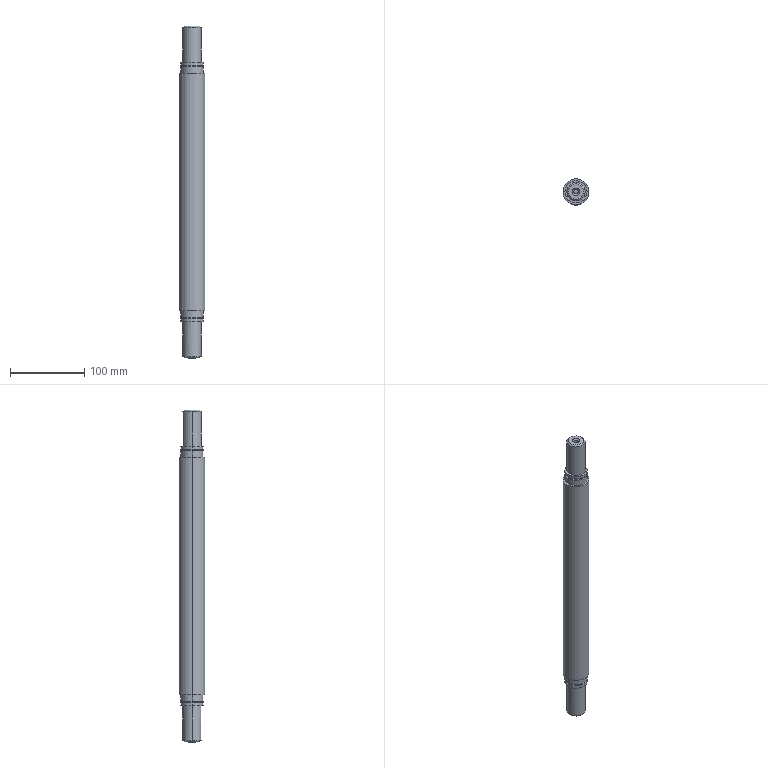Part | STEP file | Shaft 3 | 1 solid | 42 faces | box 35 x 35 x 448 mm | volume 375515 mm3 | cylinder 22 | plane 12 | cone 8 | commonest cylinder face diameters 30 x8 6 x4 25 x4 27.6 x4 35 x2
STEP:
#1=CARTESIAN_POINT('',(-17.5,0.,335.));
#2=VERTEX_POINT('',#1);
#3=CARTESIAN_POINT('',(17.5,0.,335.));
#4=VERTEX_POINT('',#3);
#5=CARTESIAN_POINT('',(0.,0.,335.));
#6=DIRECTION('',(0.,0.,-1.));
#7=DIRECTION('',(-1.,0.,0.));
#8=AXIS2_PLACEMENT_3D('',#5,#6,#7);
#9=CIRCLE('',#8,17.5);
#10=EDGE_CURVE('',#2,#4,#9,.T.);
#11=ORIENTED_EDGE('',*,*,#10,.T.);
#12=CARTESIAN_POINT('',(17.5,0.,15.));
#13=VERTEX_POINT('',#12);
#14=CARTESIAN_POINT('',(17.5,0.,350.));
#15=DIRECTION('',(0.,0.,-1.));
#16=VECTOR('',#15,1000.);
#17=LINE('',#14,#16);
#18=EDGE_CURVE('',#4,#13,#17,.T.);
#19=ORIENTED_EDGE('',*,*,#18,.T.);
#20=CARTESIAN_POINT('',(-17.5,0.,15.));
#21=VERTEX_POINT('',#20);
#22=CARTESIAN_POINT('',(0.,0.,15.));
#23=DIRECTION('',(0.,0.,1.));
#24=DIRECTION('',(-1.,0.,0.));
#25=AXIS2_PLACEMENT_3D('',#22,#23,#24);
#26=CIRCLE('',#25,17.5);
#27=EDGE_CURVE('',#13,#21,#26,.T.);
#28=ORIENTED_EDGE('',*,*,#27,.T.);
#29=CARTESIAN_POINT('',(-17.5,0.,350.));
#30=DIRECTION('',(0.,0.,-1.));
#31=VECTOR('',#30,1000.);
#32=LINE('',#29,#31);
#33=EDGE_CURVE('',#2,#21,#32,.T.);
#34=ORIENTED_EDGE('',*,*,#33,.F.);
#35=EDGE_LOOP('',(#11,#19,#28,#34));
#36=FACE_OUTER_BOUND('',#35,.T.);
#37=CARTESIAN_POINT('',(0.,0.,350.));
#38=DIRECTION('',(0.,0.,-1.));
#39=DIRECTION('',(-1.,0.,0.));
#40=AXIS2_PLACEMENT_3D('',#37,#38,#39);
#41=CYLINDRICAL_SURFACE('',#40,17.5);
#42=ADVANCED_FACE('',(#36),#41,.T.);
#43=CARTESIAN_POINT('',(15.,0.,15.));
#44=VERTEX_POINT('',#43);
#45=CARTESIAN_POINT('',(-15.,0.,15.));
#46=VERTEX_POINT('',#45);
#47=CARTESIAN_POINT('',(0.,0.,15.));
#48=DIRECTION('',(0.,0.,1.));
#49=DIRECTION('',(-1.,0.,0.));
#50=AXIS2_PLACEMENT_3D('',#47,#48,#49);
#51=CIRCLE('',#50,15.);
#52=EDGE_CURVE('',#44,#46,#51,.T.);
#53=ORIENTED_EDGE('',*,*,#52,.F.);
#54=CARTESIAN_POINT('',(15.,0.,6.));
#55=VERTEX_POINT('',#54);
#56=CARTESIAN_POINT('',(15.,0.,15.));
#57=DIRECTION('',(0.,0.,-1.));
#58=VECTOR('',#57,1000.);
#59=LINE('',#56,#58);
#60=EDGE_CURVE('',#44,#55,#59,.T.);
#61=ORIENTED_EDGE('',*,*,#60,.T.);
#62=CARTESIAN_POINT('',(-15.,0.,6.));
#63=VERTEX_POINT('',#62);
#64=CARTESIAN_POINT('',(0.,0.,6.));
#65=DIRECTION('',(0.,0.,1.));
#66=DIRECTION('',(-1.,0.,0.));
#67=AXIS2_PLACEMENT_3D('',#64,#65,#66);
#68=CIRCLE('',#67,15.);
#69=EDGE_CURVE('',#55,#63,#68,.T.);
#70=ORIENTED_EDGE('',*,*,#69,.T.);
#71=CARTESIAN_POINT('',(-15.,0.,15.));
#72=DIRECTION('',(0.,0.,-1.));
#73=VECTOR('',#72,1000.);
#74=LINE('',#71,#73);
#75=EDGE_CURVE('',#46,#63,#74,.T.);
#76=ORIENTED_EDGE('',*,*,#75,.F.);
#77=EDGE_LOOP('',(#53,#61,#70,#76));
#78=FACE_OUTER_BOUND('',#77,.T.);
#79=CARTESIAN_POINT('',(0.,0.,15.));
#80=DIRECTION('',(0.,0.,-1.));
#81=DIRECTION('',(-1.,0.,0.));
#82=AXIS2_PLACEMENT_3D('',#79,#80,#81);
#83=CYLINDRICAL_SURFACE('',#82,15.);
#84=ADVANCED_FACE('',(#78),#83,.T.);
#85=CARTESIAN_POINT('',(-15.,0.,335.));
#86=VERTEX_POINT('',#85);
#87=CARTESIAN_POINT('',(15.,0.,335.));
#88=VERTEX_POINT('',#87);
#89=CARTESIAN_POINT('',(0.,0.,335.));
#90=DIRECTION('',(0.,0.,-1.));
#91=DIRECTION('',(1.,0.,0.));
#92=AXIS2_PLACEMENT_3D('',#89,#90,#91);
#93=CIRCLE('',#92,15.);
#94=EDGE_CURVE('',#86,#88,#93,.T.);
#95=ORIENTED_EDGE('',*,*,#94,.F.);
#96=CARTESIAN_POINT('',(-15.,0.,344.));
#97=VERTEX_POINT('',#96);
#98=CARTESIAN_POINT('',(-15.,0.,335.));
#99=DIRECTION('',(0.,0.,1.));
#100=VECTOR('',#99,1000.);
#101=LINE('',#98,#100);
#102=EDGE_CURVE('',#86,#97,#101,.T.);
#103=ORIENTED_EDGE('',*,*,#102,.T.);
#104=CARTESIAN_POINT('',(15.,0.,344.));
#105=VERTEX_POINT('',#104);
#106=CARTESIAN_POINT('',(0.,0.,344.));
#107=DIRECTION('',(0.,0.,-1.));
#108=DIRECTION('',(1.,0.,0.));
#109=AXIS2_PLACEMENT_3D('',#106,#107,#108);
#110=CIRCLE('',#109,15.);
#111=EDGE_CURVE('',#97,#105,#110,.T.);
#112=ORIENTED_EDGE('',*,*,#111,.T.);
#113=CARTESIAN_POINT('',(15.,0.,335.));
#114=DIRECTION('',(0.,0.,1.));
#115=VECTOR('',#114,1000.);
#116=LINE('',#113,#115);
#117=EDGE_CURVE('',#88,#105,#116,.T.);
#118=ORIENTED_EDGE('',*,*,#117,.F.);
#119=EDGE_LOOP('',(#95,#103,#112,#118));
#120=FACE_OUTER_BOUND('',#119,.T.);
#121=CARTESIAN_POINT('',(0.,0.,335.));
#122=DIRECTION('',(0.,0.,1.));
#123=DIRECTION('',(1.,0.,0.));
#124=AXIS2_PLACEMENT_3D('',#121,#122,#123);
#125=CYLINDRICAL_SURFACE('',#124,15.);
#126=ADVANCED_FACE('',(#120),#125,.T.);
#127=CARTESIAN_POINT('',(-13.8,0.,6.));
#128=VERTEX_POINT('',#127);
#129=CARTESIAN_POINT('',(13.8,0.,6.));
#130=VERTEX_POINT('',#129);
#131=CARTESIAN_POINT('',(0.,0.,6.));
#132=DIRECTION('',(0.,0.,-1.));
#133=DIRECTION('',(-1.,0.,0.));
#134=AXIS2_PLACEMENT_3D('',#131,#132,#133);
#135=CIRCLE('',#134,13.8);
#136=EDGE_CURVE('',#128,#130,#135,.T.);
#137=ORIENTED_EDGE('',*,*,#136,.T.);
#138=CARTESIAN_POINT('',(13.8,0.,4.));
#139=VERTEX_POINT('',#138);
#140=CARTESIAN_POINT('',(13.8,0.,-31.));
#141=DIRECTION('',(0.,0.,-1.));
#142=VECTOR('',#141,1000.);
#143=LINE('',#140,#142);
#144=EDGE_CURVE('',#130,#139,#143,.T.);
#145=ORIENTED_EDGE('',*,*,#144,.T.);
#146=CARTESIAN_POINT('',(-13.8,0.,4.));
#147=VERTEX_POINT('',#146);
#148=CARTESIAN_POINT('',(0.,0.,4.));
#149=DIRECTION('',(0.,0.,1.));
#150=DIRECTION('',(-1.,0.,0.));
#151=AXIS2_PLACEMENT_3D('',#148,#149,#150);
#152=CIRCLE('',#151,13.8);
#153=EDGE_CURVE('',#139,#147,#152,.T.);
#154=ORIENTED_EDGE('',*,*,#153,.T.);
#155=CARTESIAN_POINT('',(-13.8,0.,-31.));
#156=DIRECTION('',(0.,0.,-1.));
#157=VECTOR('',#156,1000.);
#158=LINE('',#155,#157);
#159=EDGE_CURVE('',#128,#147,#158,.T.);
#160=ORIENTED_EDGE('',*,*,#159,.F.);
#161=EDGE_LOOP('',(#137,#145,#154,#160));
#162=FACE_OUTER_BOUND('',#161,.T.);
#163=CARTESIAN_POINT('',(0.,0.,-31.));
#164=DIRECTION('',(0.,0.,-1.));
#165=DIRECTION('',(-1.,0.,0.));
#166=AXIS2_PLACEMENT_3D('',#163,#164,#165);
#167=CYLINDRICAL_SURFACE('',#166,13.8);
#168=ADVANCED_FACE('',(#162),#167,.T.);
#169=CARTESIAN_POINT('',(-13.8,0.,346.));
#170=VERTEX_POINT('',#169);
#171=CARTESIAN_POINT('',(13.8,0.,346.));
#172=VERTEX_POINT('',#171);
#173=CARTESIAN_POINT('',(0.,0.,346.));
#174=DIRECTION('',(0.,0.,-1.));
#175=DIRECTION('',(-1.,0.,0.));
#176=AXIS2_PLACEMENT_3D('',#173,#174,#175);
#177=CIRCLE('',#176,13.8);
#178=EDGE_CURVE('',#170,#172,#177,.T.);
#179=ORIENTED_EDGE('',*,*,#178,.T.);
#180=CARTESIAN_POINT('',(13.8,0.,344.));
#181=VERTEX_POINT('',#180);
#182=CARTESIAN_POINT('',(13.8,0.,-31.));
#183=DIRECTION('',(0.,0.,-1.));
#184=VECTOR('',#183,1000.);
#185=LINE('',#182,#184);
#186=EDGE_CURVE('',#172,#181,#185,.T.);
#187=ORIENTED_EDGE('',*,*,#186,.T.);
#188=CARTESIAN_POINT('',(-13.8,0.,344.));
#189=VERTEX_POINT('',#188);
#190=CARTESIAN_POINT('',(0.,0.,344.));
#191=DIRECTION('',(0.,0.,1.));
#192=DIRECTION('',(-1.,0.,0.));
#193=AXIS2_PLACEMENT_3D('',#190,#191,#192);
#194=CIRCLE('',#193,13.8);
#195=EDGE_CURVE('',#181,#189,#194,.T.);
#196=ORIENTED_EDGE('',*,*,#195,.T.);
#197=CARTESIAN_POINT('',(-13.8,0.,-31.));
#198=DIRECTION('',(0.,0.,-1.));
#199=VECTOR('',#198,1000.);
#200=LINE('',#197,#199);
#201=EDGE_CURVE('',#170,#189,#200,.T.);
#202=ORIENTED_EDGE('',*,*,#201,.F.);
#203=EDGE_LOOP('',(#179,#187,#196,#202));
#204=FACE_OUTER_BOUND('',#203,.T.);
#205=CARTESIAN_POINT('',(0.,0.,-31.));
#206=DIRECTION('',(0.,0.,-1.));
#207=DIRECTION('',(-1.,0.,0.));
#208=AXIS2_PLACEMENT_3D('',#205,#206,#207);
#209=CYLINDRICAL_SURFACE('',#208,13.8);
#210=ADVANCED_FACE('',(#204),#209,.T.);
#211=CARTESIAN_POINT('',(-15.,0.,4.));
#212=VERTEX_POINT('',#211);
#213=CARTESIAN_POINT('',(15.,0.,4.));
#214=VERTEX_POINT('',#213);
#215=CARTESIAN_POINT('',(0.,0.,4.));
#216=DIRECTION('',(0.,0.,-1.));
#217=DIRECTION('',(-1.,0.,0.));
#218=AXIS2_PLACEMENT_3D('',#215,#216,#217);
#219=CIRCLE('',#218,15.);
#220=EDGE_CURVE('',#212,#214,#219,.T.);
#221=ORIENTED_EDGE('',*,*,#220,.T.);
#222=CARTESIAN_POINT('',(15.,0.,0.));
#223=VERTEX_POINT('',#222);
#224=CARTESIAN_POINT('',(15.,0.,15.));
#225=DIRECTION('',(0.,0.,-1.));
#226=VECTOR('',#225,1000.);
#227=LINE('',#224,#226);
#228=EDGE_CURVE('',#214,#223,#227,.T.);
#229=ORIENTED_EDGE('',*,*,#228,.T.);
#230=CARTESIAN_POINT('',(-15.,0.,0.));
#231=VERTEX_POINT('',#230);
#232=CARTESIAN_POINT('',(0.,0.,0.));
#233=DIRECTION('',(0.,0.,1.));
#234=DIRECTION('',(-1.,0.,0.));
#235=AXIS2_PLACEMENT_3D('',#232,#233,#234);
#236=CIRCLE('',#235,15.);
#237=EDGE_CURVE('',#223,#231,#236,.T.);
#238=ORIENTED_EDGE('',*,*,#237,.T.);
#239=CARTESIAN_POINT('',(-15.,0.,15.));
#240=DIRECTION('',(0.,0.,-1.));
#241=VECTOR('',#240,1000.);
#242=LINE('',#239,#241);
#243=EDGE_CURVE('',#212,#231,#242,.T.);
#244=ORIENTED_EDGE('',*,*,#243,.F.);
#245=EDGE_LOOP('',(#221,#229,#238,#244));
#246=FACE_OUTER_BOUND('',#245,.T.);
#247=CARTESIAN_POINT('',(0.,0.,15.));
#248=DIRECTION('',(0.,0.,-1.));
#249=DIRECTION('',(-1.,0.,0.));
#250=AXIS2_PLACEMENT_3D('',#247,#248,#249);
#251=CYLINDRICAL_SURFACE('',#250,15.);
#252=ADVANCED_FACE('',(#246),#251,.T.);
#253=CARTESIAN_POINT('',(15.,0.,346.));
#254=VERTEX_POINT('',#253);
#255=CARTESIAN_POINT('',(-15.,0.,346.));
#256=VERTEX_POINT('',#255);
#257=CARTESIAN_POINT('',(0.,0.,346.));
#258=DIRECTION('',(0.,0.,1.));
#259=DIRECTION('',(1.,0.,0.));
#260=AXIS2_PLACEMENT_3D('',#257,#258,#259);
#261=CIRCLE('',#260,15.);
#262=EDGE_CURVE('',#254,#256,#261,.T.);
#263=ORIENTED_EDGE('',*,*,#262,.T.);
#264=CARTESIAN_POINT('',(-15.,0.,350.));
#265=VERTEX_POINT('',#264);
#266=CARTESIAN_POINT('',(-15.,0.,335.));
#267=DIRECTION('',(0.,0.,1.));
#268=VECTOR('',#267,1000.);
#269=LINE('',#266,#268);
#270=EDGE_CURVE('',#256,#265,#269,.T.);
#271=ORIENTED_EDGE('',*,*,#270,.T.);
#272=CARTESIAN_POINT('',(15.,0.,350.));
#273=VERTEX_POINT('',#272);
#274=CARTESIAN_POINT('',(0.,0.,350.));
#275=DIRECTION('',(0.,0.,-1.));
#276=DIRECTION('',(1.,0.,0.));
#277=AXIS2_PLACEMENT_3D('',#274,#275,#276);
#278=CIRCLE('',#277,15.);
#279=EDGE_CURVE('',#265,#273,#278,.T.);
#280=ORIENTED_EDGE('',*,*,#279,.T.);
#281=CARTESIAN_POINT('',(15.,0.,335.));
#282=DIRECTION('',(0.,0.,1.));
#283=VECTOR('',#282,1000.);
#284=LINE('',#281,#283);
#285=EDGE_CURVE('',#254,#273,#284,.T.);
#286=ORIENTED_EDGE('',*,*,#285,.F.);
#287=EDGE_LOOP('',(#263,#271,#280,#286));
#288=FACE_OUTER_BOUND('',#287,.T.);
#289=CARTESIAN_POINT('',(0.,0.,335.));
#290=DIRECTION('',(0.,0.,1.));
#291=DIRECTION('',(1.,0.,0.));
#292=AXIS2_PLACEMENT_3D('',#289,#290,#291);
#293=CYLINDRICAL_SURFACE('',#292,15.);
#294=ADVANCED_FACE('',(#288),#293,.T.);
#295=CARTESIAN_POINT('',(0.,12.5,-47.));
#296=VERTEX_POINT('',#295);
#297=CARTESIAN_POINT('',(-12.5,0.,-47.));
#298=VERTEX_POINT('',#297);
#299=CARTESIAN_POINT('',(0.,0.,-47.));
#300=DIRECTION('',(0.,0.,1.));
#301=DIRECTION('',(1.,0.,0.));
#302=AXIS2_PLACEMENT_3D('',#299,#300,#301);
#303=CIRCLE('',#302,12.5);
#304=EDGE_CURVE('',#296,#298,#303,.T.);
#305=ORIENTED_EDGE('',*,*,#304,.T.);
#306=CARTESIAN_POINT('',(-12.5,0.,0.));
#307=VERTEX_POINT('',#306);
#308=CARTESIAN_POINT('',(-12.5,0.,-49.));
#309=DIRECTION('',(0.,0.,1.));
#310=VECTOR('',#309,1000.);
#311=LINE('',#308,#310);
#312=EDGE_CURVE('',#298,#307,#311,.T.);
#313=ORIENTED_EDGE('',*,*,#312,.T.);
#314=CARTESIAN_POINT('',(12.5,0.,0.));
#315=VERTEX_POINT('',#314);
#316=CARTESIAN_POINT('',(0.,0.,0.));
#317=DIRECTION('',(0.,0.,-1.));
#318=DIRECTION('',(1.,0.,0.));
#319=AXIS2_PLACEMENT_3D('',#316,#317,#318);
#320=CIRCLE('',#319,12.5);
#321=EDGE_CURVE('',#307,#315,#320,.T.);
#322=ORIENTED_EDGE('',*,*,#321,.T.);
#323=CARTESIAN_POINT('',(12.5,0.,-47.));
#324=VERTEX_POINT('',#323);
#325=CARTESIAN_POINT('',(12.5,0.,-49.));
#326=DIRECTION('',(0.,0.,1.));
#327=VECTOR('',#326,1000.);
#328=LINE('',#325,#327);
#329=EDGE_CURVE('',#324,#315,#328,.T.);
#330=ORIENTED_EDGE('',*,*,#329,.F.);
#331=CARTESIAN_POINT('',(0.,0.,-47.));
#332=DIRECTION('',(0.,0.,1.));
#333=DIRECTION('',(1.,0.,0.));
#334=AXIS2_PLACEMENT_3D('',#331,#332,#333);
#335=CIRCLE('',#334,12.5);
#336=EDGE_CURVE('',#324,#296,#335,.T.);
#337=ORIENTED_EDGE('',*,*,#336,.T.);
#338=EDGE_LOOP('',(#305,#313,#322,#330,#337));
#339=FACE_OUTER_BOUND('',#338,.T.);
#340=CARTESIAN_POINT('',(0.,0.,-49.));
#341=DIRECTION('',(0.,0.,1.));
#342=DIRECTION('',(1.,0.,0.));
#343=AXIS2_PLACEMENT_3D('',#340,#341,#342);
#344=CYLINDRICAL_SURFACE('',#343,12.5);
#345=ADVANCED_FACE('',(#339),#344,.T.);
#346=CARTESIAN_POINT('',(-12.5,0.,397.));
#347=VERTEX_POINT('',#346);
#348=CARTESIAN_POINT('',(12.5,0.,397.));
#349=VERTEX_POINT('',#348);
#350=CARTESIAN_POINT('',(0.,0.,397.));
#351=DIRECTION('',(0.,0.,-1.));
#352=DIRECTION('',(-1.,0.,0.));
#353=AXIS2_PLACEMENT_3D('',#350,#351,#352);
#354=CIRCLE('',#353,12.5);
#355=EDGE_CURVE('',#347,#349,#354,.T.);
#356=ORIENTED_EDGE('',*,*,#355,.T.);
#357=CARTESIAN_POINT('',(12.5,0.,350.));
#358=VERTEX_POINT('',#357);
#359=CARTESIAN_POINT('',(12.5,0.,399.));
#360=DIRECTION('',(0.,0.,-1.));
#361=VECTOR('',#360,1000.);
#362=LINE('',#359,#361);
#363=EDGE_CURVE('',#349,#358,#362,.T.);
#364=ORIENTED_EDGE('',*,*,#363,.T.);
#365=CARTESIAN_POINT('',(-12.5,0.,350.));
#366=VERTEX_POINT('',#365);
#367=CARTESIAN_POINT('',(0.,0.,350.));
#368=DIRECTION('',(0.,0.,-1.));
#369=DIRECTION('',(-1.,0.,0.));
#370=AXIS2_PLACEMENT_3D('',#367,#368,#369);
#371=CIRCLE('',#370,12.5);
#372=EDGE_CURVE('',#366,#358,#371,.T.);
#373=ORIENTED_EDGE('',*,*,#372,.F.);
#374=CARTESIAN_POINT('',(-12.5,0.,399.));
#375=DIRECTION('',(0.,0.,-1.));
#376=VECTOR('',#375,1000.);
#377=LINE('',#374,#376);
#378=EDGE_CURVE('',#347,#366,#377,.T.);
#379=ORIENTED_EDGE('',*,*,#378,.F.);
#380=EDGE_LOOP('',(#356,#364,#373,#379));
#381=FACE_OUTER_BOUND('',#380,.T.);
#382=CARTESIAN_POINT('',(0.,0.,399.));
#383=DIRECTION('',(0.,0.,-1.));
#384=DIRECTION('',(-1.,0.,0.));
#385=AXIS2_PLACEMENT_3D('',#382,#383,#384);
#386=CYLINDRICAL_SURFACE('',#385,12.5);
#387=ADVANCED_FACE('',(#381),#386,.T.);
#388=CARTESIAN_POINT('',(0.,-10.5,-49.));
#389=VERTEX_POINT('',#388);
#390=CARTESIAN_POINT('',(0.,10.5,-49.));
#391=VERTEX_POINT('',#390);
#392=CARTESIAN_POINT('',(0.,0.,-49.));
#393=DIRECTION('',(0.,0.,1.));
#394=DIRECTION('',(0.,-1.,0.));
#395=AXIS2_PLACEMENT_3D('',#392,#393,#394);
#396=CIRCLE('',#395,10.5);
#397=EDGE_CURVE('',#389,#391,#396,.T.);
#398=ORIENTED_EDGE('',*,*,#397,.T.);
#399=CARTESIAN_POINT('',(0.,12.5,-47.));
#400=DIRECTION('',(0.,0.7071,0.7071));
#401=VECTOR('',#400,1000.);
#402=LINE('',#399,#401);
#403=EDGE_CURVE('',#391,#296,#402,.T.);
#404=ORIENTED_EDGE('',*,*,#403,.T.);
#405=ORIENTED_EDGE('',*,*,#336,.F.);
#406=CARTESIAN_POINT('',(0.,-12.5,-47.));
#407=VERTEX_POINT('',#406);
#408=CARTESIAN_POINT('',(0.,0.,-47.));
#409=DIRECTION('',(0.,0.,1.));
#410=DIRECTION('',(1.,0.,0.));
#411=AXIS2_PLACEMENT_3D('',#408,#409,#410);
#412=CIRCLE('',#411,12.5);
#413=EDGE_CURVE('',#407,#324,#412,.T.);
#414=ORIENTED_EDGE('',*,*,#413,.F.);
#415=CARTESIAN_POINT('',(0.,-12.5,-47.));
#416=DIRECTION('',(0.,-0.7071,0.7071));
#417=VECTOR('',#416,1000.);
#418=LINE('',#415,#417);
#419=EDGE_CURVE('',#389,#407,#418,.T.);
#420=ORIENTED_EDGE('',*,*,#419,.F.);
#421=EDGE_LOOP('',(#398,#404,#405,#414,#420));
#422=FACE_OUTER_BOUND('',#421,.T.);
#423=CARTESIAN_POINT('',(0.,0.,-47.));
#424=DIRECTION('',(0.,0.,1.));
#425=DIRECTION('',(0.,-1.,0.));
#426=AXIS2_PLACEMENT_3D('',#423,#424,#425);
#427=CONICAL_SURFACE('',#426,12.5,0.7854);
#428=ADVANCED_FACE('',(#422),#427,.T.);
#429=CARTESIAN_POINT('',(-10.5,0.,399.));
#430=VERTEX_POINT('',#429);
#431=CARTESIAN_POINT('',(10.5,0.,399.));
#432=VERTEX_POINT('',#431);
#433=CARTESIAN_POINT('',(0.,0.,399.));
#434=DIRECTION('',(0.,0.,-1.));
#435=DIRECTION('',(-1.,0.,0.));
#436=AXIS2_PLACEMENT_3D('',#433,#434,#435);
#437=CIRCLE('',#436,10.5);
#438=EDGE_CURVE('',#430,#432,#437,.T.);
#439=ORIENTED_EDGE('',*,*,#438,.T.);
#440=CARTESIAN_POINT('',(12.5,0.,397.));
#441=DIRECTION('',(0.7071,0.,-0.7071));
#442=VECTOR('',#441,1000.);
#443=LINE('',#440,#442);
#444=EDGE_CURVE('',#432,#349,#443,.T.);
#445=ORIENTED_EDGE('',*,*,#444,.T.);
#446=ORIENTED_EDGE('',*,*,#355,.F.);
#447=CARTESIAN_POINT('',(-12.5,0.,397.));
#448=DIRECTION('',(-0.7071,0.,-0.7071));
#449=VECTOR('',#448,1000.);
#450=LINE('',#447,#449);
#451=EDGE_CURVE('',#430,#347,#450,.T.);
#452=ORIENTED_EDGE('',*,*,#451,.F.);
#453=EDGE_LOOP('',(#439,#445,#446,#452));
#454=FACE_OUTER_BOUND('',#453,.T.);
#455=CARTESIAN_POINT('',(0.,0.,397.));
#456=DIRECTION('',(0.,0.,-1.));
#457=DIRECTION('',(-1.,0.,0.));
#458=AXIS2_PLACEMENT_3D('',#455,#456,#457);
#459=CONICAL_SURFACE('',#458,12.5,0.7854);
#460=ADVANCED_FACE('',(#454),#459,.T.);
#461=CARTESIAN_POINT('',(3.,0.,-47.));
#462=VERTEX_POINT('',#461);
#463=CARTESIAN_POINT('',(-3.,0.,-47.));
#464=VERTEX_POINT('',#463);
#465=CARTESIAN_POINT('',(0.,0.,-47.));
#466=DIRECTION('',(0.,0.,-1.));
#467=DIRECTION('',(-1.,0.,0.));
#468=AXIS2_PLACEMENT_3D('',#465,#466,#467);
#469=CIRCLE('',#468,3.);
#470=EDGE_CURVE('',#462,#464,#469,.T.);
#471=ORIENTED_EDGE('',*,*,#470,.F.);
#472=CARTESIAN_POINT('',(5.,0.,-49.));
#473=VERTEX_POINT('',#472);
#474=CARTESIAN_POINT('',(5.,0.,-49.));
#475=DIRECTION('',(0.7071,0.,-0.7071));
#476=VECTOR('',#475,1000.);
#477=LINE('',#474,#476);
#478=EDGE_CURVE('',#462,#473,#477,.T.);
#479=ORIENTED_EDGE('',*,*,#478,.T.);
#480=CARTESIAN_POINT('',(-5.,0.,-49.));
#481=VERTEX_POINT('',#480);
#482=CARTESIAN_POINT('',(0.,0.,-49.));
#483=DIRECTION('',(0.,0.,1.));
#484=DIRECTION('',(-1.,0.,0.));
#485=AXIS2_PLACEMENT_3D('',#482,#483,#484);
#486=CIRCLE('',#485,5.);
#487=EDGE_CURVE('',#481,#473,#486,.T.);
#488=ORIENTED_EDGE('',*,*,#487,.F.);
#489=CARTESIAN_POINT('',(-5.,0.,-49.));
#490=DIRECTION('',(-0.7071,0.,-0.7071));
#491=VECTOR('',#490,1000.);
#492=LINE('',#489,#491);
#493=EDGE_CURVE('',#464,#481,#492,.T.);
#494=ORIENTED_EDGE('',*,*,#493,.F.);
#495=EDGE_LOOP('',(#471,#479,#488,#494));
#496=FACE_OUTER_BOUND('',#495,.T.);
#497=CARTESIAN_POINT('',(0.,0.,-49.));
#498=DIRECTION('',(0.,0.,-1.));
#499=DIRECTION('',(-1.,0.,0.));
#500=AXIS2_PLACEMENT_3D('',#497,#498,#499);
#501=CONICAL_SURFACE('',#500,5.,0.7854);
#502=ADVANCED_FACE('',(#496),#501,.F.);
#503=CARTESIAN_POINT('',(-3.,0.,397.));
#504=VERTEX_POINT('',#503);
#505=CARTESIAN_POINT('',(3.,0.,397.));
#506=VERTEX_POINT('',#505);
#507=CARTESIAN_POINT('',(0.,0.,397.));
#508=DIRECTION('',(0.,0.,1.));
#509=DIRECTION('',(1.,0.,0.));
#510=AXIS2_PLACEMENT_3D('',#507,#508,#509);
#511=CIRCLE('',#510,3.);
#512=EDGE_CURVE('',#504,#506,#511,.T.);
#513=ORIENTED_EDGE('',*,*,#512,.F.);
#514=CARTESIAN_POINT('',(-5.,0.,399.));
#515=VERTEX_POINT('',#514);
#516=CARTESIAN_POINT('',(-5.,0.,399.));
#517=DIRECTION('',(-0.7071,0.,0.7071));
#518=VECTOR('',#517,1000.);
#519=LINE('',#516,#518);
#520=EDGE_CURVE('',#504,#515,#519,.T.);
#521=ORIENTED_EDGE('',*,*,#520,.T.);
#522=CARTESIAN_POINT('',(5.,0.,399.));
#523=VERTEX_POINT('',#522);
#524=CARTESIAN_POINT('',(0.,0.,399.));
#525=DIRECTION('',(0.,0.,-1.));
#526=DIRECTION('',(1.,0.,0.));
#527=AXIS2_PLACEMENT_3D('',#524,#525,#526);
#528=CIRCLE('',#527,5.);
#529=EDGE_CURVE('',#523,#515,#528,.T.);
#530=ORIENTED_EDGE('',*,*,#529,.F.);
#531=CARTESIAN_POINT('',(5.,0.,399.));
#532=DIRECTION('',(0.7071,0.,0.7071));
#533=VECTOR('',#532,1000.);
#534=LINE('',#531,#533);
#535=EDGE_CURVE('',#506,#523,#534,.T.);
#536=ORIENTED_EDGE('',*,*,#535,.F.);
#537=EDGE_LOOP('',(#513,#521,#530,#536));
#538=FACE_OUTER_BOUND('',#537,.T.);
#539=CARTESIAN_POINT('',(0.,0.,399.));
#540=DIRECTION('',(0.,0.,1.));
#541=DIRECTION('',(1.,0.,0.));
#542=AXIS2_PLACEMENT_3D('',#539,#540,#541);
#543=CONICAL_SURFACE('',#542,5.,0.7854);
#544=ADVANCED_FACE('',(#538),#543,.F.);
#545=CARTESIAN_POINT('',(3.,0.,-34.));
#546=VERTEX_POINT('',#545);
#547=CARTESIAN_POINT('',(-3.,0.,-34.));
#548=VERTEX_POINT('',#547);
#549=CARTESIAN_POINT('',(0.,0.,-34.));
#550=DIRECTION('',(0.,0.,-1.));
#551=DIRECTION('',(-1.,0.,0.));
#552=AXIS2_PLACEMENT_3D('',#549,#550,#551);
#553=CIRCLE('',#552,3.);
#554=EDGE_CURVE('',#546,#548,#553,.T.);
#555=ORIENTED_EDGE('',*,*,#554,.F.);
#556=CARTESIAN_POINT('',(3.,0.,-34.));
#557=DIRECTION('',(0.,0.,-1.));
#558=VECTOR('',#557,1000.);
#559=LINE('',#556,#558);
#560=EDGE_CURVE('',#546,#462,#559,.T.);
#561=ORIENTED_EDGE('',*,*,#560,.T.);
#562=ORIENTED_EDGE('',*,*,#470,.T.);
#563=CARTESIAN_POINT('',(-3.,0.,-34.));
#564=DIRECTION('',(0.,0.,-1.));
#565=VECTOR('',#564,1000.);
#566=LINE('',#563,#565);
#567=EDGE_CURVE('',#548,#464,#566,.T.);
#568=ORIENTED_EDGE('',*,*,#567,.F.);
#569=EDGE_LOOP('',(#555,#561,#562,#568));
#570=FACE_OUTER_BOUND('',#569,.T.);
#571=CARTESIAN_POINT('',(0.,0.,-34.));
#572=DIRECTION('',(0.,0.,-1.));
#573=DIRECTION('',(-1.,0.,0.));
#574=AXIS2_PLACEMENT_3D('',#571,#572,#573);
#575=CYLINDRICAL_SURFACE('',#574,3.);
#576=ADVANCED_FACE('',(#570),#575,.F.);
#577=CARTESIAN_POINT('',(-3.,0.,384.));
#578=VERTEX_POINT('',#577);
#579=CARTESIAN_POINT('',(3.,0.,384.));
#580=VERTEX_POINT('',#579);
#581=CARTESIAN_POINT('',(0.,0.,384.));
#582=DIRECTION('',(0.,0.,1.));
#583=DIRECTION('',(1.,0.,0.));
#584=AXIS2_PLACEMENT_3D('',#581,#582,#583);
#585=CIRCLE('',#584,3.);
#586=EDGE_CURVE('',#578,#580,#585,.T.);
#587=ORIENTED_EDGE('',*,*,#586,.F.);
#588=CARTESIAN_POINT('',(-3.,0.,384.));
#589=DIRECTION('',(0.,0.,1.));
#590=VECTOR('',#589,1000.);
#591=LINE('',#588,#590);
#592=EDGE_CURVE('',#578,#504,#591,.T.);
#593=ORIENTED_EDGE('',*,*,#592,.T.);
#594=ORIENTED_EDGE('',*,*,#512,.T.);
#595=CARTESIAN_POINT('',(3.,0.,384.));
#596=DIRECTION('',(0.,0.,1.));
#597=VECTOR('',#596,1000.);
#598=LINE('',#595,#597);
#599=EDGE_CURVE('',#580,#506,#598,.T.);
#600=ORIENTED_EDGE('',*,*,#599,.F.);
#601=EDGE_LOOP('',(#587,#593,#594,#600));
#602=FACE_OUTER_BOUND('',#601,.T.);
#603=CARTESIAN_POINT('',(0.,0.,384.));
#604=DIRECTION('',(0.,0.,1.));
#605=DIRECTION('',(1.,0.,0.));
#606=AXIS2_PLACEMENT_3D('',#603,#604,#605);
#607=CYLINDRICAL_SURFACE('',#606,3.);
#608=ADVANCED_FACE('',(#602),#607,.F.);
#609=ORIENTED_EDGE('',*,*,#18,.F.);
#610=CARTESIAN_POINT('',(0.,0.,335.));
#611=DIRECTION('',(0.,0.,-1.));
#612=DIRECTION('',(-1.,0.,0.));
#613=AXIS2_PLACEMENT_3D('',#610,#611,#612);
#614=CIRCLE('',#613,17.5);
#615=EDGE_CURVE('',#4,#2,#614,.T.);
#616=ORIENTED_EDGE('',*,*,#615,.T.);
#617=ORIENTED_EDGE('',*,*,#33,.T.);
#618=CARTESIAN_POINT('',(0.,0.,15.));
#619=DIRECTION('',(0.,0.,1.));
#620=DIRECTION('',(-1.,0.,0.));
#621=AXIS2_PLACEMENT_3D('',#618,#619,#620);
#622=CIRCLE('',#621,17.5);
#623=EDGE_CURVE('',#21,#13,#622,.T.);
#624=ORIENTED_EDGE('',*,*,#623,.T.);
#625=EDGE_LOOP('',(#609,#616,#617,#624));
#626=FACE_OUTER_BOUND('',#625,.T.);
#627=CARTESIAN_POINT('',(0.,0.,350.));
#628=DIRECTION('',(0.,0.,-1.));
#629=DIRECTION('',(-1.,0.,0.));
#630=AXIS2_PLACEMENT_3D('',#627,#628,#629);
#631=CYLINDRICAL_SURFACE('',#630,17.5);
#632=ADVANCED_FACE('',(#626),#631,.T.);
#633=ORIENTED_EDGE('',*,*,#623,.F.);
#634=ORIENTED_EDGE('',*,*,#27,.F.);
#635=EDGE_LOOP('',(#633,#634));
#636=FACE_OUTER_BOUND('',#635,.T.);
#637=CARTESIAN_POINT('',(0.,0.,15.));
#638=DIRECTION('',(0.,0.,1.));
#639=DIRECTION('',(-1.,0.,0.));
#640=AXIS2_PLACEMENT_3D('',#637,#638,#639);
#641=CIRCLE('',#640,15.);
#642=EDGE_CURVE('',#46,#44,#641,.T.);
#643=ORIENTED_EDGE('',*,*,#642,.T.);
#644=ORIENTED_EDGE('',*,*,#52,.T.);
#645=EDGE_LOOP('',(#643,#644));
#646=FACE_BOUND('',#645,.T.);
#647=CARTESIAN_POINT('',(0.,0.,15.));
#648=DIRECTION('',(0.,0.,-1.));
#649=DIRECTION('',(-1.,0.,0.));
#650=AXIS2_PLACEMENT_3D('',#647,#648,#649);
#651=PLANE('',#650);
#652=ADVANCED_FACE('',(#636,#646),#651,.T.);
#653=ORIENTED_EDGE('',*,*,#10,.F.);
#654=ORIENTED_EDGE('',*,*,#615,.F.);
#655=EDGE_LOOP('',(#653,#654));
#656=FACE_OUTER_BOUND('',#655,.T.);
#657=CARTESIAN_POINT('',(0.,0.,335.));
#658=DIRECTION('',(0.,0.,-1.));
#659=DIRECTION('',(1.,0.,0.));
#660=AXIS2_PLACEMENT_3D('',#657,#658,#659);
#661=CIRCLE('',#660,15.);
#662=EDGE_CURVE('',#88,#86,#661,.T.);
#663=ORIENTED_EDGE('',*,*,#662,.T.);
#664=ORIENTED_EDGE('',*,*,#94,.T.);
#665=EDGE_LOOP('',(#663,#664));
#666=FACE_BOUND('',#665,.T.);
#667=CARTESIAN_POINT('',(0.,0.,335.));
#668=DIRECTION('',(0.,0.,1.));
#669=DIRECTION('',(1.,0.,0.));
#670=AXIS2_PLACEMENT_3D('',#667,#668,#669);
#671=PLANE('',#670);
#672=ADVANCED_FACE('',(#656,#666),#671,.T.);
#673=ORIENTED_EDGE('',*,*,#60,.F.);
#674=ORIENTED_EDGE('',*,*,#642,.F.);
#675=ORIENTED_EDGE('',*,*,#75,.T.);
#676=CARTESIAN_POINT('',(0.,0.,6.));
#677=DIRECTION('',(0.,0.,1.));
#678=DIRECTION('',(-1.,0.,0.));
#679=AXIS2_PLACEMENT_3D('',#676,#677,#678);
#680=CIRCLE('',#679,15.);
#681=EDGE_CURVE('',#63,#55,#680,.T.);
#682=ORIENTED_EDGE('',*,*,#681,.T.);
#683=EDGE_LOOP('',(#673,#674,#675,#682));
#684=FACE_OUTER_BOUND('',#683,.T.);
#685=CARTESIAN_POINT('',(0.,0.,15.));
#686=DIRECTION('',(0.,0.,-1.));
#687=DIRECTION('',(-1.,0.,0.));
#688=AXIS2_PLACEMENT_3D('',#685,#686,#687);
#689=CYLINDRICAL_SURFACE('',#688,15.);
#690=ADVANCED_FACE('',(#684),#689,.T.);
#691=ORIENTED_EDGE('',*,*,#102,.F.);
#692=ORIENTED_EDGE('',*,*,#662,.F.);
#693=ORIENTED_EDGE('',*,*,#117,.T.);
#694=CARTESIAN_POINT('',(0.,0.,344.));
#695=DIRECTION('',(0.,0.,-1.));
#696=DIRECTION('',(1.,0.,0.));
#697=AXIS2_PLACEMENT_3D('',#694,#695,#696);
#698=CIRCLE('',#697,15.);
#699=EDGE_CURVE('',#105,#97,#698,.T.);
#700=ORIENTED_EDGE('',*,*,#699,.T.);
#701=EDGE_LOOP('',(#691,#692,#693,#700));
#702=FACE_OUTER_BOUND('',#701,.T.);
#703=CARTESIAN_POINT('',(0.,0.,335.));
#704=DIRECTION('',(0.,0.,1.));
#705=DIRECTION('',(1.,0.,0.));
#706=AXIS2_PLACEMENT_3D('',#703,#704,#705);
#707=CYLINDRICAL_SURFACE('',#706,15.);
#708=ADVANCED_FACE('',(#702),#707,.T.);
#709=ORIENTED_EDGE('',*,*,#136,.F.);
#710=CARTESIAN_POINT('',(0.,0.,6.));
#711=DIRECTION('',(0.,0.,-1.));
#712=DIRECTION('',(-1.,0.,0.));
#713=AXIS2_PLACEMENT_3D('',#710,#711,#712);
#714=CIRCLE('',#713,13.8);
#715=EDGE_CURVE('',#130,#128,#714,.T.);
#716=ORIENTED_EDGE('',*,*,#715,.F.);
#717=EDGE_LOOP('',(#709,#716));
#718=FACE_BOUND('',#717,.T.);
#719=ORIENTED_EDGE('',*,*,#681,.F.);
#720=ORIENTED_EDGE('',*,*,#69,.F.);
#721=EDGE_LOOP('',(#719,#720));
#722=FACE_OUTER_BOUND('',#721,.T.);
#723=CARTESIAN_POINT('',(-16.8,0.,6.));
#724=DIRECTION('',(0.,0.,1.));
#725=DIRECTION('',(1.,0.,0.));
#726=AXIS2_PLACEMENT_3D('',#723,#724,#725);
#727=PLANE('',#726);
#728=ADVANCED_FACE('',(#718,#722),#727,.F.);
#729=CARTESIAN_POINT('',(0.,0.,344.));
#730=DIRECTION('',(0.,0.,1.));
#731=DIRECTION('',(-1.,0.,0.));
#732=AXIS2_PLACEMENT_3D('',#729,#730,#731);
#733=CIRCLE('',#732,13.8);
#734=EDGE_CURVE('',#189,#181,#733,.T.);
#735=ORIENTED_EDGE('',*,*,#734,.F.);
#736=ORIENTED_EDGE('',*,*,#195,.F.);
#737=EDGE_LOOP('',(#735,#736));
#738=FACE_BOUND('',#737,.T.);
#739=ORIENTED_EDGE('',*,*,#699,.F.);
#740=ORIENTED_EDGE('',*,*,#111,.F.);
#741=EDGE_LOOP('',(#739,#740));
#742=FACE_OUTER_BOUND('',#741,.T.);
#743=CARTESIAN_POINT('',(-16.8,0.,344.));
#744=DIRECTION('',(0.,0.,-1.));
#745=DIRECTION('',(-1.,0.,0.));
#746=AXIS2_PLACEMENT_3D('',#743,#744,#745);
#747=PLANE('',#746);
#748=ADVANCED_FACE('',(#738,#742),#747,.F.);
#749=ORIENTED_EDGE('',*,*,#144,.F.);
#750=ORIENTED_EDGE('',*,*,#715,.T.);
#751=ORIENTED_EDGE('',*,*,#159,.T.);
#752=CARTESIAN_POINT('',(0.,0.,4.));
#753=DIRECTION('',(0.,0.,1.));
#754=DIRECTION('',(-1.,0.,0.));
#755=AXIS2_PLACEMENT_3D('',#752,#753,#754);
#756=CIRCLE('',#755,13.8);
#757=EDGE_CURVE('',#147,#139,#756,.T.);
#758=ORIENTED_EDGE('',*,*,#757,.T.);
#759=EDGE_LOOP('',(#749,#750,#751,#758));
#760=FACE_OUTER_BOUND('',#759,.T.);
#761=CARTESIAN_POINT('',(0.,0.,-31.));
#762=DIRECTION('',(0.,0.,-1.));
#763=DIRECTION('',(-1.,0.,0.));
#764=AXIS2_PLACEMENT_3D('',#761,#762,#763);
#765=CYLINDRICAL_SURFACE('',#764,13.8);
#766=ADVANCED_FACE('',(#760),#765,.T.);
#767=ORIENTED_EDGE('',*,*,#186,.F.);
#768=CARTESIAN_POINT('',(0.,0.,346.));
#769=DIRECTION('',(0.,0.,-1.));
#770=DIRECTION('',(-1.,0.,0.));
#771=AXIS2_PLACEMENT_3D('',#768,#769,#770);
#772=CIRCLE('',#771,13.8);
#773=EDGE_CURVE('',#172,#170,#772,.T.);
#774=ORIENTED_EDGE('',*,*,#773,.T.);
#775=ORIENTED_EDGE('',*,*,#201,.T.);
#776=ORIENTED_EDGE('',*,*,#734,.T.);
#777=EDGE_LOOP('',(#767,#774,#775,#776));
#778=FACE_OUTER_BOUND('',#777,.T.);
#779=CARTESIAN_POINT('',(0.,0.,-31.));
#780=DIRECTION('',(0.,0.,-1.));
#781=DIRECTION('',(-1.,0.,0.));
#782=AXIS2_PLACEMENT_3D('',#779,#780,#781);
#783=CYLINDRICAL_SURFACE('',#782,13.8);
#784=ADVANCED_FACE('',(#778),#783,.T.);
#785=ORIENTED_EDGE('',*,*,#757,.F.);
#786=ORIENTED_EDGE('',*,*,#153,.F.);
#787=EDGE_LOOP('',(#785,#786));
#788=FACE_BOUND('',#787,.T.);
#789=ORIENTED_EDGE('',*,*,#220,.F.);
#790=CARTESIAN_POINT('',(0.,0.,4.));
#791=DIRECTION('',(0.,0.,-1.));
#792=DIRECTION('',(-1.,0.,0.));
#793=AXIS2_PLACEMENT_3D('',#790,#791,#792);
#794=CIRCLE('',#793,15.);
#795=EDGE_CURVE('',#214,#212,#794,.T.);
#796=ORIENTED_EDGE('',*,*,#795,.F.);
#797=EDGE_LOOP('',(#789,#796));
#798=FACE_OUTER_BOUND('',#797,.T.);
#799=CARTESIAN_POINT('',(-16.8,0.,4.));
#800=DIRECTION('',(0.,0.,-1.));
#801=DIRECTION('',(-1.,0.,0.));
#802=AXIS2_PLACEMENT_3D('',#799,#800,#801);
#803=PLANE('',#802);
#804=ADVANCED_FACE('',(#788,#798),#803,.F.);
#805=ORIENTED_EDGE('',*,*,#178,.F.);
#806=ORIENTED_EDGE('',*,*,#773,.F.);
#807=EDGE_LOOP('',(#805,#806));
#808=FACE_BOUND('',#807,.T.);
#809=ORIENTED_EDGE('',*,*,#262,.F.);
#810=CARTESIAN_POINT('',(0.,0.,346.));
#811=DIRECTION('',(0.,0.,1.));
#812=DIRECTION('',(1.,0.,0.));
#813=AXIS2_PLACEMENT_3D('',#810,#811,#812);
#814=CIRCLE('',#813,15.);
#815=EDGE_CURVE('',#256,#254,#814,.T.);
#816=ORIENTED_EDGE('',*,*,#815,.F.);
#817=EDGE_LOOP('',(#809,#816));
#818=FACE_OUTER_BOUND('',#817,.T.);
#819=CARTESIAN_POINT('',(-16.8,0.,346.));
#820=DIRECTION('',(0.,0.,1.));
#821=DIRECTION('',(1.,0.,0.));
#822=AXIS2_PLACEMENT_3D('',#819,#820,#821);
#823=PLANE('',#822);
#824=ADVANCED_FACE('',(#808,#818),#823,.F.);
#825=ORIENTED_EDGE('',*,*,#228,.F.);
#826=ORIENTED_EDGE('',*,*,#795,.T.);
#827=ORIENTED_EDGE('',*,*,#243,.T.);
#828=CARTESIAN_POINT('',(0.,0.,0.));
#829=DIRECTION('',(0.,0.,1.));
#830=DIRECTION('',(-1.,0.,0.));
#831=AXIS2_PLACEMENT_3D('',#828,#829,#830);
#832=CIRCLE('',#831,15.);
#833=EDGE_CURVE('',#231,#223,#832,.T.);
#834=ORIENTED_EDGE('',*,*,#833,.T.);
#835=EDGE_LOOP('',(#825,#826,#827,#834));
#836=FACE_OUTER_BOUND('',#835,.T.);
#837=CARTESIAN_POINT('',(0.,0.,15.));
#838=DIRECTION('',(0.,0.,-1.));
#839=DIRECTION('',(-1.,0.,0.));
#840=AXIS2_PLACEMENT_3D('',#837,#838,#839);
#841=CYLINDRICAL_SURFACE('',#840,15.);
#842=ADVANCED_FACE('',(#836),#841,.T.);
#843=ORIENTED_EDGE('',*,*,#270,.F.);
#844=ORIENTED_EDGE('',*,*,#815,.T.);
#845=ORIENTED_EDGE('',*,*,#285,.T.);
#846=CARTESIAN_POINT('',(0.,0.,350.));
#847=DIRECTION('',(0.,0.,-1.));
#848=DIRECTION('',(1.,0.,0.));
#849=AXIS2_PLACEMENT_3D('',#846,#847,#848);
#850=CIRCLE('',#849,15.);
#851=EDGE_CURVE('',#273,#265,#850,.T.);
#852=ORIENTED_EDGE('',*,*,#851,.T.);
#853=EDGE_LOOP('',(#843,#844,#845,#852));
#854=FACE_OUTER_BOUND('',#853,.T.);
#855=CARTESIAN_POINT('',(0.,0.,335.));
#856=DIRECTION('',(0.,0.,1.));
#857=DIRECTION('',(1.,0.,0.));
#858=AXIS2_PLACEMENT_3D('',#855,#856,#857);
#859=CYLINDRICAL_SURFACE('',#858,15.);
#860=ADVANCED_FACE('',(#854),#859,.T.);
#861=ORIENTED_EDGE('',*,*,#833,.F.);
#862=ORIENTED_EDGE('',*,*,#237,.F.);
#863=EDGE_LOOP('',(#861,#862));
#864=FACE_OUTER_BOUND('',#863,.T.);
#865=CARTESIAN_POINT('',(0.,0.,0.));
#866=DIRECTION('',(0.,0.,-1.));
#867=DIRECTION('',(1.,0.,0.));
#868=AXIS2_PLACEMENT_3D('',#865,#866,#867);
#869=CIRCLE('',#868,12.5);
#870=EDGE_CURVE('',#315,#307,#869,.T.);
#871=ORIENTED_EDGE('',*,*,#870,.F.);
#872=ORIENTED_EDGE('',*,*,#321,.F.);
#873=EDGE_LOOP('',(#871,#872));
#874=FACE_BOUND('',#873,.T.);
#875=CARTESIAN_POINT('',(0.,0.,0.));
#876=DIRECTION('',(0.,0.,1.));
#877=DIRECTION('',(1.,0.,0.));
#878=AXIS2_PLACEMENT_3D('',#875,#876,#877);
#879=PLANE('',#878);
#880=ADVANCED_FACE('',(#864,#874),#879,.F.);
#881=ORIENTED_EDGE('',*,*,#851,.F.);
#882=ORIENTED_EDGE('',*,*,#279,.F.);
#883=EDGE_LOOP('',(#881,#882));
#884=FACE_OUTER_BOUND('',#883,.T.);
#885=ORIENTED_EDGE('',*,*,#372,.T.);
#886=CARTESIAN_POINT('',(0.,0.,350.));
#887=DIRECTION('',(0.,0.,-1.));
#888=DIRECTION('',(-1.,0.,0.));
#889=AXIS2_PLACEMENT_3D('',#886,#887,#888);
#890=CIRCLE('',#889,12.5);
#891=EDGE_CURVE('',#358,#366,#890,.T.);
#892=ORIENTED_EDGE('',*,*,#891,.T.);
#893=EDGE_LOOP('',(#885,#892));
#894=FACE_BOUND('',#893,.T.);
#895=CARTESIAN_POINT('',(0.,0.,350.));
#896=DIRECTION('',(0.,0.,1.));
#897=DIRECTION('',(1.,0.,0.));
#898=AXIS2_PLACEMENT_3D('',#895,#896,#897);
#899=PLANE('',#898);
#900=ADVANCED_FACE('',(#884,#894),#899,.T.);
#901=ORIENTED_EDGE('',*,*,#312,.F.);
#902=CARTESIAN_POINT('',(0.,0.,-47.));
#903=DIRECTION('',(0.,0.,1.));
#904=DIRECTION('',(1.,0.,0.));
#905=AXIS2_PLACEMENT_3D('',#902,#903,#904);
#906=CIRCLE('',#905,12.5);
#907=EDGE_CURVE('',#298,#407,#906,.T.);
#908=ORIENTED_EDGE('',*,*,#907,.T.);
#909=ORIENTED_EDGE('',*,*,#413,.T.);
#910=ORIENTED_EDGE('',*,*,#329,.T.);
#911=ORIENTED_EDGE('',*,*,#870,.T.);
#912=EDGE_LOOP('',(#901,#908,#909,#910,#911));
#913=FACE_OUTER_BOUND('',#912,.T.);
#914=CARTESIAN_POINT('',(0.,0.,-49.));
#915=DIRECTION('',(0.,0.,1.));
#916=DIRECTION('',(1.,0.,0.));
#917=AXIS2_PLACEMENT_3D('',#914,#915,#916);
#918=CYLINDRICAL_SURFACE('',#917,12.5);
#919=ADVANCED_FACE('',(#913),#918,.T.);
#920=ORIENTED_EDGE('',*,*,#363,.F.);
#921=CARTESIAN_POINT('',(0.,0.,397.));
#922=DIRECTION('',(0.,0.,-1.));
#923=DIRECTION('',(-1.,0.,0.));
#924=AXIS2_PLACEMENT_3D('',#921,#922,#923);
#925=CIRCLE('',#924,12.5);
#926=EDGE_CURVE('',#349,#347,#925,.T.);
#927=ORIENTED_EDGE('',*,*,#926,.T.);
#928=ORIENTED_EDGE('',*,*,#378,.T.);
#929=ORIENTED_EDGE('',*,*,#891,.F.);
#930=EDGE_LOOP('',(#920,#927,#928,#929));
#931=FACE_OUTER_BOUND('',#930,.T.);
#932=CARTESIAN_POINT('',(0.,0.,399.));
#933=DIRECTION('',(0.,0.,-1.));
#934=DIRECTION('',(-1.,0.,0.));
#935=AXIS2_PLACEMENT_3D('',#932,#933,#934);
#936=CYLINDRICAL_SURFACE('',#935,12.5);
#937=ADVANCED_FACE('',(#931),#936,.T.);
#938=ORIENTED_EDGE('',*,*,#403,.F.);
#939=CARTESIAN_POINT('',(0.,0.,-49.));
#940=DIRECTION('',(0.,0.,1.));
#941=DIRECTION('',(0.,-1.,0.));
#942=AXIS2_PLACEMENT_3D('',#939,#940,#941);
#943=CIRCLE('',#942,10.5);
#944=EDGE_CURVE('',#391,#389,#943,.T.);
#945=ORIENTED_EDGE('',*,*,#944,.T.);
#946=ORIENTED_EDGE('',*,*,#419,.T.);
#947=ORIENTED_EDGE('',*,*,#907,.F.);
#948=ORIENTED_EDGE('',*,*,#304,.F.);
#949=EDGE_LOOP('',(#938,#945,#946,#947,#948));
#950=FACE_OUTER_BOUND('',#949,.T.);
#951=CARTESIAN_POINT('',(0.,0.,-47.));
#952=DIRECTION('',(0.,0.,1.));
#953=DIRECTION('',(0.,-1.,0.));
#954=AXIS2_PLACEMENT_3D('',#951,#952,#953);
#955=CONICAL_SURFACE('',#954,12.5,0.7854);
#956=ADVANCED_FACE('',(#950),#955,.T.);
#957=ORIENTED_EDGE('',*,*,#444,.F.);
#958=CARTESIAN_POINT('',(0.,0.,399.));
#959=DIRECTION('',(0.,0.,-1.));
#960=DIRECTION('',(-1.,0.,0.));
#961=AXIS2_PLACEMENT_3D('',#958,#959,#960);
#962=CIRCLE('',#961,10.5);
#963=EDGE_CURVE('',#432,#430,#962,.T.);
#964=ORIENTED_EDGE('',*,*,#963,.T.);
#965=ORIENTED_EDGE('',*,*,#451,.T.);
#966=ORIENTED_EDGE('',*,*,#926,.F.);
#967=EDGE_LOOP('',(#957,#964,#965,#966));
#968=FACE_OUTER_BOUND('',#967,.T.);
#969=CARTESIAN_POINT('',(0.,0.,397.));
#970=DIRECTION('',(0.,0.,-1.));
#971=DIRECTION('',(-1.,0.,0.));
#972=AXIS2_PLACEMENT_3D('',#969,#970,#971);
#973=CONICAL_SURFACE('',#972,12.5,0.7854);
#974=ADVANCED_FACE('',(#968),#973,.T.);
#975=ORIENTED_EDGE('',*,*,#397,.F.);
#976=ORIENTED_EDGE('',*,*,#944,.F.);
#977=EDGE_LOOP('',(#975,#976));
#978=FACE_OUTER_BOUND('',#977,.T.);
#979=ORIENTED_EDGE('',*,*,#487,.T.);
#980=CARTESIAN_POINT('',(0.,0.,-49.));
#981=DIRECTION('',(0.,0.,1.));
#982=DIRECTION('',(-1.,0.,0.));
#983=AXIS2_PLACEMENT_3D('',#980,#981,#982);
#984=CIRCLE('',#983,5.);
#985=EDGE_CURVE('',#473,#481,#984,.T.);
#986=ORIENTED_EDGE('',*,*,#985,.T.);
#987=EDGE_LOOP('',(#979,#986));
#988=FACE_BOUND('',#987,.T.);
#989=CARTESIAN_POINT('',(0.,0.,-49.));
#990=DIRECTION('',(0.,0.,-1.));
#991=DIRECTION('',(-1.,0.,0.));
#992=AXIS2_PLACEMENT_3D('',#989,#990,#991);
#993=PLANE('',#992);
#994=ADVANCED_FACE('',(#978,#988),#993,.T.);
#995=ORIENTED_EDGE('',*,*,#438,.F.);
#996=ORIENTED_EDGE('',*,*,#963,.F.);
#997=EDGE_LOOP('',(#995,#996));
#998=FACE_OUTER_BOUND('',#997,.T.);
#999=ORIENTED_EDGE('',*,*,#529,.T.);
#1000=CARTESIAN_POINT('',(0.,0.,399.));
#1001=DIRECTION('',(0.,0.,-1.));
#1002=DIRECTION('',(1.,0.,0.));
#1003=AXIS2_PLACEMENT_3D('',#1000,#1001,#1002);
#1004=CIRCLE('',#1003,5.);
#1005=EDGE_CURVE('',#515,#523,#1004,.T.);
#1006=ORIENTED_EDGE('',*,*,#1005,.T.);
#1007=EDGE_LOOP('',(#999,#1006));
#1008=FACE_BOUND('',#1007,.T.);
#1009=CARTESIAN_POINT('',(0.,0.,399.));
#1010=DIRECTION('',(0.,0.,1.));
#1011=DIRECTION('',(1.,0.,0.));
#1012=AXIS2_PLACEMENT_3D('',#1009,#1010,#1011);
#1013=PLANE('',#1012);
#1014=ADVANCED_FACE('',(#998,#1008),#1013,.T.);
#1015=ORIENTED_EDGE('',*,*,#478,.F.);
#1016=CARTESIAN_POINT('',(0.,0.,-47.));
#1017=DIRECTION('',(0.,0.,-1.));
#1018=DIRECTION('',(-1.,0.,0.));
#1019=AXIS2_PLACEMENT_3D('',#1016,#1017,#1018);
#1020=CIRCLE('',#1019,3.);
#1021=EDGE_CURVE('',#464,#462,#1020,.T.);
#1022=ORIENTED_EDGE('',*,*,#1021,.F.);
#1023=ORIENTED_EDGE('',*,*,#493,.T.);
#1024=ORIENTED_EDGE('',*,*,#985,.F.);
#1025=EDGE_LOOP('',(#1015,#1022,#1023,#1024));
#1026=FACE_OUTER_BOUND('',#1025,.T.);
#1027=CARTESIAN_POINT('',(0.,0.,-49.));
#1028=DIRECTION('',(0.,0.,-1.));
#1029=DIRECTION('',(-1.,0.,0.));
#1030=AXIS2_PLACEMENT_3D('',#1027,#1028,#1029);
#1031=CONICAL_SURFACE('',#1030,5.,0.7854);
#1032=ADVANCED_FACE('',(#1026),#1031,.F.);
#1033=ORIENTED_EDGE('',*,*,#520,.F.);
#1034=CARTESIAN_POINT('',(0.,0.,397.));
#1035=DIRECTION('',(0.,0.,1.));
#1036=DIRECTION('',(1.,0.,0.));
#1037=AXIS2_PLACEMENT_3D('',#1034,#1035,#1036);
#1038=CIRCLE('',#1037,3.);
#1039=EDGE_CURVE('',#506,#504,#1038,.T.);
#1040=ORIENTED_EDGE('',*,*,#1039,.F.);
#1041=ORIENTED_EDGE('',*,*,#535,.T.);
#1042=ORIENTED_EDGE('',*,*,#1005,.F.);
#1043=EDGE_LOOP('',(#1033,#1040,#1041,#1042));
#1044=FACE_OUTER_BOUND('',#1043,.T.);
#1045=CARTESIAN_POINT('',(0.,0.,399.));
#1046=DIRECTION('',(0.,0.,1.));
#1047=DIRECTION('',(1.,0.,0.));
#1048=AXIS2_PLACEMENT_3D('',#1045,#1046,#1047);
#1049=CONICAL_SURFACE('',#1048,5.,0.7854);
#1050=ADVANCED_FACE('',(#1044),#1049,.F.);
#1051=ORIENTED_EDGE('',*,*,#560,.F.);
#1052=CARTESIAN_POINT('',(0.,0.,-34.));
#1053=DIRECTION('',(0.,0.,-1.));
#1054=DIRECTION('',(-1.,0.,0.));
#1055=AXIS2_PLACEMENT_3D('',#1052,#1053,#1054);
#1056=CIRCLE('',#1055,3.);
#1057=EDGE_CURVE('',#548,#546,#1056,.T.);
#1058=ORIENTED_EDGE('',*,*,#1057,.F.);
#1059=ORIENTED_EDGE('',*,*,#567,.T.);
#1060=ORIENTED_EDGE('',*,*,#1021,.T.);
#1061=EDGE_LOOP('',(#1051,#1058,#1059,#1060));
#1062=FACE_OUTER_BOUND('',#1061,.T.);
#1063=CARTESIAN_POINT('',(0.,0.,-34.));
#1064=DIRECTION('',(0.,0.,-1.));
#1065=DIRECTION('',(-1.,0.,0.));
#1066=AXIS2_PLACEMENT_3D('',#1063,#1064,#1065);
#1067=CYLINDRICAL_SURFACE('',#1066,3.);
#1068=ADVANCED_FACE('',(#1062),#1067,.F.);
#1069=ORIENTED_EDGE('',*,*,#592,.F.);
#1070=CARTESIAN_POINT('',(0.,0.,384.));
#1071=DIRECTION('',(0.,0.,1.));
#1072=DIRECTION('',(1.,0.,0.));
#1073=AXIS2_PLACEMENT_3D('',#1070,#1071,#1072);
#1074=CIRCLE('',#1073,3.);
#1075=EDGE_CURVE('',#580,#578,#1074,.T.);
#1076=ORIENTED_EDGE('',*,*,#1075,.F.);
#1077=ORIENTED_EDGE('',*,*,#599,.T.);
#1078=ORIENTED_EDGE('',*,*,#1039,.T.);
#1079=EDGE_LOOP('',(#1069,#1076,#1077,#1078));
#1080=FACE_OUTER_BOUND('',#1079,.T.);
#1081=CARTESIAN_POINT('',(0.,0.,384.));
#1082=DIRECTION('',(0.,0.,1.));
#1083=DIRECTION('',(1.,0.,0.));
#1084=AXIS2_PLACEMENT_3D('',#1081,#1082,#1083);
#1085=CYLINDRICAL_SURFACE('',#1084,3.);
#1086=ADVANCED_FACE('',(#1080),#1085,.F.);
#1087=ORIENTED_EDGE('',*,*,#1057,.T.);
#1088=ORIENTED_EDGE('',*,*,#554,.T.);
#1089=EDGE_LOOP('',(#1087,#1088));
#1090=FACE_OUTER_BOUND('',#1089,.T.);
#1091=CARTESIAN_POINT('',(0.,0.,-34.));
#1092=DIRECTION('',(0.,0.,-1.));
#1093=DIRECTION('',(-1.,0.,0.));
#1094=AXIS2_PLACEMENT_3D('',#1091,#1092,#1093);
#1095=PLANE('',#1094);
#1096=ADVANCED_FACE('',(#1090),#1095,.T.);
#1097=ORIENTED_EDGE('',*,*,#1075,.T.);
#1098=ORIENTED_EDGE('',*,*,#586,.T.);
#1099=EDGE_LOOP('',(#1097,#1098));
#1100=FACE_OUTER_BOUND('',#1099,.T.);
#1101=CARTESIAN_POINT('',(0.,0.,384.));
#1102=DIRECTION('',(0.,0.,1.));
#1103=DIRECTION('',(1.,0.,0.));
#1104=AXIS2_PLACEMENT_3D('',#1101,#1102,#1103);
#1105=PLANE('',#1104);
#1106=ADVANCED_FACE('',(#1100),#1105,.T.);
#1107=CLOSED_SHELL('',(#42,#84,#126,#168,#210,#252,#294,#345,#387,#428,#460,#502,#544,#576,#608,#632,#652,#672,#690,#708,#728,#748,#766,#784,#804,#824,#842,#860,#880,#900,#919,#937,#956,#974,#994,#1014,#1032,#1050,#1068,#1086,#1096,#1106));
#1108=MANIFOLD_SOLID_BREP('',#1107);
#1109=CARTESIAN_POINT('',(0.,0.,0.));
#1110=DIRECTION('',(0.,0.,1.));
#1111=DIRECTION('',(1.,0.,0.));
#1112=AXIS2_PLACEMENT_3D('',#1109,#1110,#1111);
#1113=(LENGTH_UNIT()NAMED_UNIT(*)SI_UNIT(.MILLI.,.METRE.));
#1114=UNCERTAINTY_MEASURE_WITH_UNIT(LENGTH_MEASURE(0.00001),#1113,'','');
#1115=(NAMED_UNIT(*)PLANE_ANGLE_UNIT()SI_UNIT($,.RADIAN.));
#1116=(NAMED_UNIT(*)SI_UNIT($,.STERADIAN.)SOLID_ANGLE_UNIT());
#1117=(GEOMETRIC_REPRESENTATION_CONTEXT(3)GLOBAL_UNCERTAINTY_ASSIGNED_CONTEXT((#1114))GLOBAL_UNIT_ASSIGNED_CONTEXT((#1113,#1115,#1116))REPRESENTATION_CONTEXT('',''));
#1118=ADVANCED_BREP_SHAPE_REPRESENTATION('',(#1108,#1112),#1117);